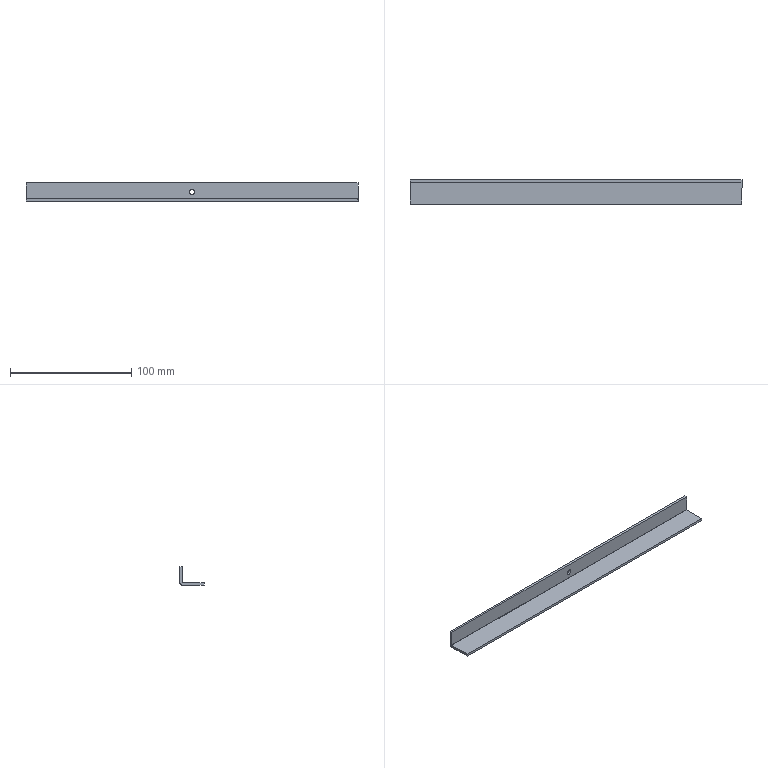Part | SolidWorks | features BaseBody 1 | 1 solid | 12 faces | box 274 x 20 x 15 mm | volume 17798 mm3 | plane 8 | cylinder 4 | commonest cylinder face diameters 4.2 x3 0.2 x1
STEP:
#1=CARTESIAN_POINT('',(0.,8.,3.4));
#2=VERTEX_POINT('',#1);
#3=CARTESIAN_POINT('',(0.,8.,7.6));
#4=VERTEX_POINT('',#3);
#5=CARTESIAN_POINT('',(0.,8.,5.5));
#6=DIRECTION('',(0.,1.,0.));
#7=DIRECTION('',(0.,0.,1.));
#8=AXIS2_PLACEMENT_3D('',#5,#6,#7);
#9=CIRCLE('',#8,2.1);
#10=EDGE_CURVE('',#2,#4,#9,.T.);
#11=ORIENTED_EDGE('',*,*,#10,.F.);
#12=CARTESIAN_POINT('',(0.,10.,3.4));
#13=VERTEX_POINT('',#12);
#14=CARTESIAN_POINT('',(0.,10.,3.4));
#15=DIRECTION('',(0.,1.,0.));
#16=VECTOR('',#15,1000.);
#17=LINE('',#14,#16);
#18=EDGE_CURVE('',#2,#13,#17,.T.);
#19=ORIENTED_EDGE('',*,*,#18,.T.);
#20=CARTESIAN_POINT('',(0.,10.,7.6));
#21=VERTEX_POINT('',#20);
#22=CARTESIAN_POINT('',(0.,10.,5.5));
#23=DIRECTION('',(0.,1.,0.));
#24=DIRECTION('',(0.,0.,1.));
#25=AXIS2_PLACEMENT_3D('',#22,#23,#24);
#26=CIRCLE('',#25,2.1);
#27=EDGE_CURVE('',#13,#21,#26,.T.);
#28=ORIENTED_EDGE('',*,*,#27,.T.);
#29=CARTESIAN_POINT('',(0.,10.,7.6));
#30=DIRECTION('',(0.,1.,0.));
#31=VECTOR('',#30,1000.);
#32=LINE('',#29,#31);
#33=EDGE_CURVE('',#4,#21,#32,.T.);
#34=ORIENTED_EDGE('',*,*,#33,.F.);
#35=EDGE_LOOP('',(#11,#19,#28,#34));
#36=FACE_OUTER_BOUND('',#35,.T.);
#37=CARTESIAN_POINT('',(0.,10.,5.5));
#38=DIRECTION('',(0.,1.,0.));
#39=DIRECTION('',(0.,0.,1.));
#40=AXIS2_PLACEMENT_3D('',#37,#38,#39);
#41=CYLINDRICAL_SURFACE('',#40,2.1);
#42=ADVANCED_FACE('',(#36),#41,.F.);
#43=CARTESIAN_POINT('',(137.,-10.,-2.));
#44=VERTEX_POINT('',#43);
#45=CARTESIAN_POINT('',(137.,7.9,-2.));
#46=VERTEX_POINT('',#45);
#47=CARTESIAN_POINT('',(137.,0.,-2.));
#48=DIRECTION('',(0.,1.,0.));
#49=VECTOR('',#48,1000.);
#50=LINE('',#47,#49);
#51=EDGE_CURVE('',#44,#46,#50,.T.);
#52=ORIENTED_EDGE('',*,*,#51,.F.);
#53=CARTESIAN_POINT('',(-137.,-10.,-2.));
#54=VERTEX_POINT('',#53);
#55=CARTESIAN_POINT('',(0.,-10.,-2.));
#56=DIRECTION('',(1.,0.,0.));
#57=VECTOR('',#56,1000.);
#58=LINE('',#55,#57);
#59=EDGE_CURVE('',#54,#44,#58,.T.);
#60=ORIENTED_EDGE('',*,*,#59,.F.);
#61=CARTESIAN_POINT('',(-137.,7.9,-2.));
#62=VERTEX_POINT('',#61);
#63=CARTESIAN_POINT('',(-137.,0.,-2.));
#64=DIRECTION('',(0.,-1.,0.));
#65=VECTOR('',#64,1000.);
#66=LINE('',#63,#65);
#67=EDGE_CURVE('',#62,#54,#66,.T.);
#68=ORIENTED_EDGE('',*,*,#67,.F.);
#69=CARTESIAN_POINT('',(0.,7.9,-2.));
#70=DIRECTION('',(-1.,0.,0.));
#71=VECTOR('',#70,1000.);
#72=LINE('',#69,#71);
#73=EDGE_CURVE('',#46,#62,#72,.T.);
#74=ORIENTED_EDGE('',*,*,#73,.F.);
#75=EDGE_LOOP('',(#52,#60,#68,#74));
#76=FACE_OUTER_BOUND('',#75,.T.);
#77=CARTESIAN_POINT('',(0.,0.,-2.));
#78=DIRECTION('',(0.,0.,1.));
#79=DIRECTION('',(1.,0.,0.));
#80=AXIS2_PLACEMENT_3D('',#77,#78,#79);
#81=PLANE('',#80);
#82=ADVANCED_FACE('',(#76),#81,.F.);
#83=CARTESIAN_POINT('',(-137.,10.,0.1));
#84=VERTEX_POINT('',#83);
#85=CARTESIAN_POINT('',(137.,10.,0.1));
#86=VERTEX_POINT('',#85);
#87=CARTESIAN_POINT('',(-137.,10.,0.1));
#88=DIRECTION('',(1.,0.,0.));
#89=VECTOR('',#88,1000.);
#90=LINE('',#87,#89);
#91=EDGE_CURVE('',#84,#86,#90,.T.);
#92=ORIENTED_EDGE('',*,*,#91,.T.);
#93=CARTESIAN_POINT('',(137.,7.9,0.1));
#94=DIRECTION('',(-1.,0.,0.));
#95=DIRECTION('',(0.,-1.,0.));
#96=AXIS2_PLACEMENT_3D('',#93,#94,#95);
#97=CIRCLE('',#96,2.1);
#98=EDGE_CURVE('',#86,#46,#97,.T.);
#99=ORIENTED_EDGE('',*,*,#98,.T.);
#100=ORIENTED_EDGE('',*,*,#73,.T.);
#101=CARTESIAN_POINT('',(-137.,7.9,0.1));
#102=DIRECTION('',(1.,0.,0.));
#103=DIRECTION('',(0.,-1.,0.));
#104=AXIS2_PLACEMENT_3D('',#101,#102,#103);
#105=CIRCLE('',#104,2.1);
#106=EDGE_CURVE('',#62,#84,#105,.T.);
#107=ORIENTED_EDGE('',*,*,#106,.T.);
#108=EDGE_LOOP('',(#92,#99,#100,#107));
#109=FACE_OUTER_BOUND('',#108,.T.);
#110=CARTESIAN_POINT('',(-137.,7.9,0.1));
#111=DIRECTION('',(-1.,0.,0.));
#112=DIRECTION('',(0.,-1.,0.));
#113=AXIS2_PLACEMENT_3D('',#110,#111,#112);
#114=CYLINDRICAL_SURFACE('',#113,2.1);
#115=ADVANCED_FACE('',(#109),#114,.T.);
#116=CARTESIAN_POINT('',(137.,-10.,0.));
#117=VERTEX_POINT('',#116);
#118=CARTESIAN_POINT('',(137.,-10.,-2.));
#119=DIRECTION('',(0.,0.,-1.));
#120=VECTOR('',#119,1000.);
#121=LINE('',#118,#120);
#122=EDGE_CURVE('',#117,#44,#121,.T.);
#123=ORIENTED_EDGE('',*,*,#122,.T.);
#124=ORIENTED_EDGE('',*,*,#51,.T.);
#125=ORIENTED_EDGE('',*,*,#98,.F.);
#126=CARTESIAN_POINT('',(137.,10.,13.));
#127=VERTEX_POINT('',#126);
#128=CARTESIAN_POINT('',(137.,10.,0.));
#129=DIRECTION('',(0.,0.,1.));
#130=VECTOR('',#129,1000.);
#131=LINE('',#128,#130);
#132=EDGE_CURVE('',#86,#127,#131,.T.);
#133=ORIENTED_EDGE('',*,*,#132,.T.);
#134=CARTESIAN_POINT('',(137.,8.,13.));
#135=VERTEX_POINT('',#134);
#136=CARTESIAN_POINT('',(137.,10.,13.));
#137=DIRECTION('',(0.,1.,0.));
#138=VECTOR('',#137,1000.);
#139=LINE('',#136,#138);
#140=EDGE_CURVE('',#135,#127,#139,.T.);
#141=ORIENTED_EDGE('',*,*,#140,.F.);
#142=CARTESIAN_POINT('',(137.,8.,0.1));
#143=VERTEX_POINT('',#142);
#144=CARTESIAN_POINT('',(137.,8.,0.));
#145=DIRECTION('',(0.,0.,1.));
#146=VECTOR('',#145,1000.);
#147=LINE('',#144,#146);
#148=EDGE_CURVE('',#143,#135,#147,.T.);
#149=ORIENTED_EDGE('',*,*,#148,.F.);
#150=CARTESIAN_POINT('',(137.,7.9,0.));
#151=VERTEX_POINT('',#150);
#152=CARTESIAN_POINT('',(137.,7.9,0.1));
#153=DIRECTION('',(-1.,0.,0.));
#154=DIRECTION('',(0.,-1.,0.));
#155=AXIS2_PLACEMENT_3D('',#152,#153,#154);
#156=CIRCLE('',#155,0.1);
#157=EDGE_CURVE('',#143,#151,#156,.T.);
#158=ORIENTED_EDGE('',*,*,#157,.T.);
#159=CARTESIAN_POINT('',(137.,10.,0.));
#160=DIRECTION('',(0.,-1.,0.));
#161=VECTOR('',#160,1000.);
#162=LINE('',#159,#161);
#163=EDGE_CURVE('',#151,#117,#162,.T.);
#164=ORIENTED_EDGE('',*,*,#163,.T.);
#165=EDGE_LOOP('',(#123,#124,#125,#133,#141,#149,#158,#164));
#166=FACE_OUTER_BOUND('',#165,.T.);
#167=CARTESIAN_POINT('',(137.,10.,-2.));
#168=DIRECTION('',(1.,0.,0.));
#169=DIRECTION('',(0.,1.,0.));
#170=AXIS2_PLACEMENT_3D('',#167,#168,#169);
#171=PLANE('',#170);
#172=ADVANCED_FACE('',(#166),#171,.T.);
#173=ORIENTED_EDGE('',*,*,#59,.T.);
#174=ORIENTED_EDGE('',*,*,#122,.F.);
#175=CARTESIAN_POINT('',(-137.,-10.,0.));
#176=VERTEX_POINT('',#175);
#177=CARTESIAN_POINT('',(-137.,-10.,0.));
#178=DIRECTION('',(-1.,0.,0.));
#179=VECTOR('',#178,1000.);
#180=LINE('',#177,#179);
#181=EDGE_CURVE('',#117,#176,#180,.T.);
#182=ORIENTED_EDGE('',*,*,#181,.T.);
#183=CARTESIAN_POINT('',(-137.,-10.,-2.));
#184=DIRECTION('',(0.,0.,-1.));
#185=VECTOR('',#184,1000.);
#186=LINE('',#183,#185);
#187=EDGE_CURVE('',#176,#54,#186,.T.);
#188=ORIENTED_EDGE('',*,*,#187,.T.);
#189=EDGE_LOOP('',(#173,#174,#182,#188));
#190=FACE_OUTER_BOUND('',#189,.T.);
#191=CARTESIAN_POINT('',(-137.,-10.,-2.));
#192=DIRECTION('',(0.,-1.,0.));
#193=DIRECTION('',(1.,0.,0.));
#194=AXIS2_PLACEMENT_3D('',#191,#192,#193);
#195=PLANE('',#194);
#196=ADVANCED_FACE('',(#190),#195,.T.);
#197=ORIENTED_EDGE('',*,*,#67,.T.);
#198=ORIENTED_EDGE('',*,*,#187,.F.);
#199=CARTESIAN_POINT('',(-137.,7.9,0.));
#200=VERTEX_POINT('',#199);
#201=CARTESIAN_POINT('',(-137.,10.,0.));
#202=DIRECTION('',(0.,1.,0.));
#203=VECTOR('',#202,1000.);
#204=LINE('',#201,#203);
#205=EDGE_CURVE('',#176,#200,#204,.T.);
#206=ORIENTED_EDGE('',*,*,#205,.T.);
#207=CARTESIAN_POINT('',(-137.,8.,0.1));
#208=VERTEX_POINT('',#207);
#209=CARTESIAN_POINT('',(-137.,7.9,0.1));
#210=DIRECTION('',(1.,0.,0.));
#211=DIRECTION('',(0.,-1.,0.));
#212=AXIS2_PLACEMENT_3D('',#209,#210,#211);
#213=CIRCLE('',#212,0.1);
#214=EDGE_CURVE('',#200,#208,#213,.T.);
#215=ORIENTED_EDGE('',*,*,#214,.T.);
#216=CARTESIAN_POINT('',(-137.,8.,13.));
#217=VERTEX_POINT('',#216);
#218=CARTESIAN_POINT('',(-137.,8.,13.));
#219=DIRECTION('',(0.,0.,-1.));
#220=VECTOR('',#219,1000.);
#221=LINE('',#218,#220);
#222=EDGE_CURVE('',#217,#208,#221,.T.);
#223=ORIENTED_EDGE('',*,*,#222,.F.);
#224=CARTESIAN_POINT('',(-137.,10.,13.));
#225=VERTEX_POINT('',#224);
#226=CARTESIAN_POINT('',(-137.,10.,13.));
#227=DIRECTION('',(0.,-1.,0.));
#228=VECTOR('',#227,1000.);
#229=LINE('',#226,#228);
#230=EDGE_CURVE('',#225,#217,#229,.T.);
#231=ORIENTED_EDGE('',*,*,#230,.F.);
#232=CARTESIAN_POINT('',(-137.,10.,0.));
#233=DIRECTION('',(0.,0.,-1.));
#234=VECTOR('',#233,1000.);
#235=LINE('',#232,#234);
#236=EDGE_CURVE('',#225,#84,#235,.T.);
#237=ORIENTED_EDGE('',*,*,#236,.T.);
#238=ORIENTED_EDGE('',*,*,#106,.F.);
#239=EDGE_LOOP('',(#197,#198,#206,#215,#223,#231,#237,#238));
#240=FACE_OUTER_BOUND('',#239,.T.);
#241=CARTESIAN_POINT('',(-137.,10.,-2.));
#242=DIRECTION('',(-1.,0.,0.));
#243=DIRECTION('',(0.,-1.,0.));
#244=AXIS2_PLACEMENT_3D('',#241,#242,#243);
#245=PLANE('',#244);
#246=ADVANCED_FACE('',(#240),#245,.T.);
#247=ORIENTED_EDGE('',*,*,#236,.F.);
#248=CARTESIAN_POINT('',(0.,10.,13.));
#249=DIRECTION('',(-1.,0.,0.));
#250=VECTOR('',#249,1000.);
#251=LINE('',#248,#250);
#252=EDGE_CURVE('',#127,#225,#251,.T.);
#253=ORIENTED_EDGE('',*,*,#252,.F.);
#254=ORIENTED_EDGE('',*,*,#132,.F.);
#255=ORIENTED_EDGE('',*,*,#91,.F.);
#256=EDGE_LOOP('',(#247,#253,#254,#255));
#257=FACE_OUTER_BOUND('',#256,.T.);
#258=CARTESIAN_POINT('',(0.,10.,5.5));
#259=DIRECTION('',(0.,1.,0.));
#260=DIRECTION('',(0.,0.,1.));
#261=AXIS2_PLACEMENT_3D('',#258,#259,#260);
#262=CIRCLE('',#261,2.1);
#263=EDGE_CURVE('',#21,#13,#262,.T.);
#264=ORIENTED_EDGE('',*,*,#263,.F.);
#265=ORIENTED_EDGE('',*,*,#27,.F.);
#266=EDGE_LOOP('',(#264,#265));
#267=FACE_BOUND('',#266,.T.);
#268=CARTESIAN_POINT('',(0.,10.,0.));
#269=DIRECTION('',(0.,-1.,0.));
#270=DIRECTION('',(0.,0.,-1.));
#271=AXIS2_PLACEMENT_3D('',#268,#269,#270);
#272=PLANE('',#271);
#273=ADVANCED_FACE('',(#257,#267),#272,.F.);
#274=ORIENTED_EDGE('',*,*,#205,.F.);
#275=ORIENTED_EDGE('',*,*,#181,.F.);
#276=ORIENTED_EDGE('',*,*,#163,.F.);
#277=CARTESIAN_POINT('',(0.,7.9,0.));
#278=DIRECTION('',(-1.,0.,0.));
#279=VECTOR('',#278,1000.);
#280=LINE('',#277,#279);
#281=EDGE_CURVE('',#151,#200,#280,.T.);
#282=ORIENTED_EDGE('',*,*,#281,.T.);
#283=EDGE_LOOP('',(#274,#275,#276,#282));
#284=FACE_OUTER_BOUND('',#283,.T.);
#285=CARTESIAN_POINT('',(0.,0.,0.));
#286=DIRECTION('',(0.,0.,1.));
#287=DIRECTION('',(1.,0.,0.));
#288=AXIS2_PLACEMENT_3D('',#285,#286,#287);
#289=PLANE('',#288);
#290=ADVANCED_FACE('',(#284),#289,.T.);
#291=ORIENTED_EDGE('',*,*,#140,.T.);
#292=ORIENTED_EDGE('',*,*,#252,.T.);
#293=ORIENTED_EDGE('',*,*,#230,.T.);
#294=CARTESIAN_POINT('',(137.,8.,13.));
#295=DIRECTION('',(-1.,0.,0.));
#296=VECTOR('',#295,1000.);
#297=LINE('',#294,#296);
#298=EDGE_CURVE('',#135,#217,#297,.T.);
#299=ORIENTED_EDGE('',*,*,#298,.F.);
#300=EDGE_LOOP('',(#291,#292,#293,#299));
#301=FACE_OUTER_BOUND('',#300,.T.);
#302=CARTESIAN_POINT('',(137.,10.,13.));
#303=DIRECTION('',(0.,0.,-1.));
#304=DIRECTION('',(0.,1.,0.));
#305=AXIS2_PLACEMENT_3D('',#302,#303,#304);
#306=PLANE('',#305);
#307=ADVANCED_FACE('',(#301),#306,.F.);
#308=ORIENTED_EDGE('',*,*,#18,.F.);
#309=CARTESIAN_POINT('',(0.,8.,5.5));
#310=DIRECTION('',(0.,1.,0.));
#311=DIRECTION('',(0.,0.,1.));
#312=AXIS2_PLACEMENT_3D('',#309,#310,#311);
#313=CIRCLE('',#312,2.1);
#314=EDGE_CURVE('',#4,#2,#313,.T.);
#315=ORIENTED_EDGE('',*,*,#314,.F.);
#316=ORIENTED_EDGE('',*,*,#33,.T.);
#317=ORIENTED_EDGE('',*,*,#263,.T.);
#318=EDGE_LOOP('',(#308,#315,#316,#317));
#319=FACE_OUTER_BOUND('',#318,.T.);
#320=CARTESIAN_POINT('',(0.,10.,5.5));
#321=DIRECTION('',(0.,1.,0.));
#322=DIRECTION('',(0.,0.,1.));
#323=AXIS2_PLACEMENT_3D('',#320,#321,#322);
#324=CYLINDRICAL_SURFACE('',#323,2.1);
#325=ADVANCED_FACE('',(#319),#324,.F.);
#326=ORIENTED_EDGE('',*,*,#157,.F.);
#327=CARTESIAN_POINT('',(-137.,8.,0.1));
#328=DIRECTION('',(1.,0.,0.));
#329=VECTOR('',#328,1000.);
#330=LINE('',#327,#329);
#331=EDGE_CURVE('',#208,#143,#330,.T.);
#332=ORIENTED_EDGE('',*,*,#331,.F.);
#333=ORIENTED_EDGE('',*,*,#214,.F.);
#334=ORIENTED_EDGE('',*,*,#281,.F.);
#335=EDGE_LOOP('',(#326,#332,#333,#334));
#336=FACE_OUTER_BOUND('',#335,.T.);
#337=CARTESIAN_POINT('',(-137.,7.9,0.1));
#338=DIRECTION('',(-1.,0.,0.));
#339=DIRECTION('',(0.,-1.,0.));
#340=AXIS2_PLACEMENT_3D('',#337,#338,#339);
#341=CYLINDRICAL_SURFACE('',#340,0.1);
#342=ADVANCED_FACE('',(#336),#341,.F.);
#343=ORIENTED_EDGE('',*,*,#148,.T.);
#344=ORIENTED_EDGE('',*,*,#298,.T.);
#345=ORIENTED_EDGE('',*,*,#222,.T.);
#346=ORIENTED_EDGE('',*,*,#331,.T.);
#347=EDGE_LOOP('',(#343,#344,#345,#346));
#348=FACE_OUTER_BOUND('',#347,.T.);
#349=ORIENTED_EDGE('',*,*,#314,.T.);
#350=ORIENTED_EDGE('',*,*,#10,.T.);
#351=EDGE_LOOP('',(#349,#350));
#352=FACE_BOUND('',#351,.T.);
#353=CARTESIAN_POINT('',(0.,8.,0.));
#354=DIRECTION('',(0.,-1.,0.));
#355=DIRECTION('',(0.,0.,-1.));
#356=AXIS2_PLACEMENT_3D('',#353,#354,#355);
#357=PLANE('',#356);
#358=ADVANCED_FACE('',(#348,#352),#357,.T.);
#359=CLOSED_SHELL('',(#42,#82,#115,#172,#196,#246,#273,#290,#307,#325,#342,#358));
#360=MANIFOLD_SOLID_BREP('',#359);
#361=CARTESIAN_POINT('',(0.,0.,0.));
#362=DIRECTION('',(0.,0.,1.));
#363=DIRECTION('',(1.,0.,0.));
#364=AXIS2_PLACEMENT_3D('',#361,#362,#363);
#365=(LENGTH_UNIT()NAMED_UNIT(*)SI_UNIT(.MILLI.,.METRE.));
#366=UNCERTAINTY_MEASURE_WITH_UNIT(LENGTH_MEASURE(0.00001),#365,'','');
#367=(NAMED_UNIT(*)PLANE_ANGLE_UNIT()SI_UNIT($,.RADIAN.));
#368=(NAMED_UNIT(*)SI_UNIT($,.STERADIAN.)SOLID_ANGLE_UNIT());
#369=(GEOMETRIC_REPRESENTATION_CONTEXT(3)GLOBAL_UNCERTAINTY_ASSIGNED_CONTEXT((#366))GLOBAL_UNIT_ASSIGNED_CONTEXT((#365,#367,#368))REPRESENTATION_CONTEXT('',''));
#370=ADVANCED_BREP_SHAPE_REPRESENTATION('',(#360,#364),#369);